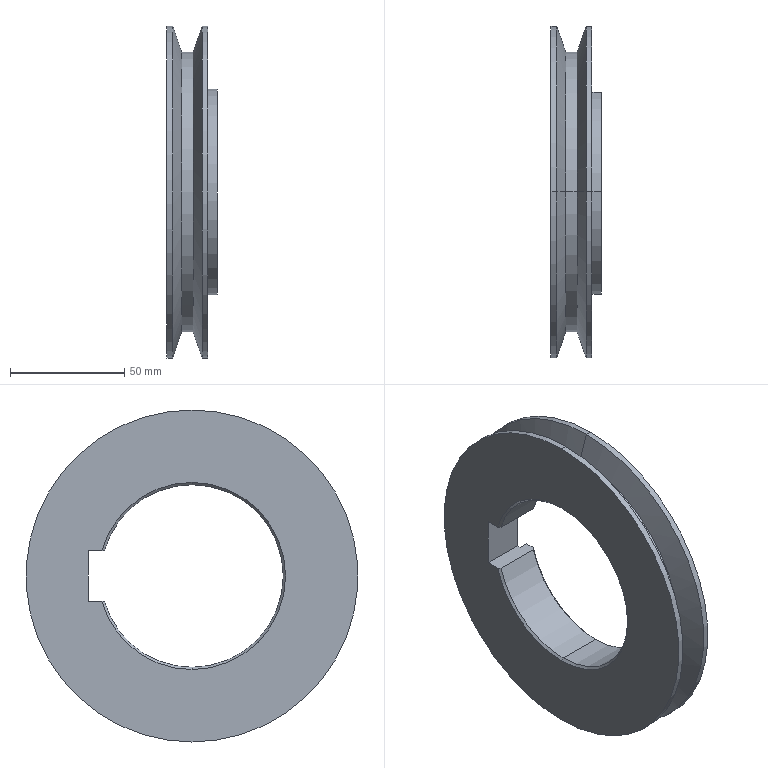Part | NX | features BREP 1 | 1 solid | 28 faces | box 22 x 145.5 x 145.5 mm | volume 167430 mm3 | cylinder 12 | cone 10 | plane 6 | commonest cylinder face diameters 145.5 x4 80 x3 90 x3 122.6 x2
STEP:
#1=CARTESIAN_POINT('',(1.,0.,-40.));
#2=VERTEX_POINT('',#1);
#3=CARTESIAN_POINT('',(1.,0.,40.));
#4=VERTEX_POINT('',#3);
#5=CARTESIAN_POINT('',(1.,0.,0.));
#6=DIRECTION('',(-1.,0.,0.));
#7=DIRECTION('',(0.,0.,-1.));
#8=AXIS2_PLACEMENT_3D('',#5,#6,#7);
#9=CIRCLE('',#8,40.);
#10=EDGE_CURVE('',#2,#4,#9,.T.);
#11=ORIENTED_EDGE('',*,*,#10,.F.);
#12=CARTESIAN_POINT('',(0.,0.,-41.));
#13=VERTEX_POINT('',#12);
#14=CARTESIAN_POINT('',(1.,0.,-40.));
#15=DIRECTION('',(-0.7071,0.,-0.7071));
#16=VECTOR('',#15,1000.);
#17=LINE('',#14,#16);
#18=EDGE_CURVE('',#2,#13,#17,.T.);
#19=ORIENTED_EDGE('',*,*,#18,.T.);
#20=CARTESIAN_POINT('',(0.,0.,41.));
#21=VERTEX_POINT('',#20);
#22=CARTESIAN_POINT('',(0.,0.,0.));
#23=DIRECTION('',(1.,0.,0.));
#24=DIRECTION('',(0.,0.,-1.));
#25=AXIS2_PLACEMENT_3D('',#22,#23,#24);
#26=CIRCLE('',#25,41.);
#27=EDGE_CURVE('',#21,#13,#26,.T.);
#28=ORIENTED_EDGE('',*,*,#27,.F.);
#29=CARTESIAN_POINT('',(1.,0.,40.));
#30=DIRECTION('',(-0.7071,0.,0.7071));
#31=VECTOR('',#30,1000.);
#32=LINE('',#29,#31);
#33=EDGE_CURVE('',#4,#21,#32,.T.);
#34=ORIENTED_EDGE('',*,*,#33,.F.);
#35=EDGE_LOOP('',(#11,#19,#28,#34));
#36=FACE_BOUND('',#35,.T.);
#37=CARTESIAN_POINT('',(1.,0.,0.));
#38=DIRECTION('',(-1.,0.,0.));
#39=DIRECTION('',(0.,0.,-1.));
#40=AXIS2_PLACEMENT_3D('',#37,#38,#39);
#41=CONICAL_SURFACE('',#40,40.,0.7854);
#42=ADVANCED_FACE('',(#36),#41,.F.);
#43=CARTESIAN_POINT('',(1.,38.458,11.));
#44=VERTEX_POINT('',#43);
#45=CARTESIAN_POINT('',(1.,0.,0.));
#46=DIRECTION('',(-1.,0.,0.));
#47=DIRECTION('',(0.,0.,-1.));
#48=AXIS2_PLACEMENT_3D('',#45,#46,#47);
#49=CIRCLE('',#48,40.);
#50=EDGE_CURVE('',#4,#44,#49,.T.);
#51=ORIENTED_EDGE('',*,*,#50,.F.);
#52=ORIENTED_EDGE('',*,*,#33,.T.);
#53=CARTESIAN_POINT('',(0.,39.497,11.));
#54=VERTEX_POINT('',#53);
#55=CARTESIAN_POINT('',(0.,0.,0.));
#56=DIRECTION('',(1.,0.,0.));
#57=DIRECTION('',(0.,0.,-1.));
#58=AXIS2_PLACEMENT_3D('',#55,#56,#57);
#59=CIRCLE('',#58,41.);
#60=EDGE_CURVE('',#54,#21,#59,.T.);
#61=ORIENTED_EDGE('',*,*,#60,.F.);
#62=CARTESIAN_POINT('',(1.,38.458,11.));
#63=CARTESIAN_POINT('',(0.6668,38.804,11.));
#64=CARTESIAN_POINT('',(0.3335,39.151,11.));
#65=CARTESIAN_POINT('',(0.,39.497,11.));
#66=B_SPLINE_CURVE_WITH_KNOTS('',3,(#62,#63,#64,#65),.UNSPECIFIED.,.F.,.F.,(4,4),(0.,1.),.PIECEWISE_BEZIER_KNOTS.);
#67=EDGE_CURVE('',#44,#54,#66,.T.);
#68=ORIENTED_EDGE('',*,*,#67,.F.);
#69=EDGE_LOOP('',(#51,#52,#61,#68));
#70=FACE_BOUND('',#69,.T.);
#71=CARTESIAN_POINT('',(1.,0.,0.));
#72=DIRECTION('',(-1.,0.,0.));
#73=DIRECTION('',(0.,0.,-1.));
#74=AXIS2_PLACEMENT_3D('',#71,#72,#73);
#75=CONICAL_SURFACE('',#74,40.,0.7854);
#76=ADVANCED_FACE('',(#70),#75,.F.);
#77=CARTESIAN_POINT('',(21.,0.,40.));
#78=VERTEX_POINT('',#77);
#79=CARTESIAN_POINT('',(21.,0.,-40.));
#80=VERTEX_POINT('',#79);
#81=CARTESIAN_POINT('',(21.,0.,0.));
#82=DIRECTION('',(1.,0.,0.));
#83=DIRECTION('',(0.,0.,1.));
#84=AXIS2_PLACEMENT_3D('',#81,#82,#83);
#85=CIRCLE('',#84,40.);
#86=EDGE_CURVE('',#78,#80,#85,.T.);
#87=ORIENTED_EDGE('',*,*,#86,.F.);
#88=CARTESIAN_POINT('',(22.,0.,41.));
#89=VERTEX_POINT('',#88);
#90=CARTESIAN_POINT('',(22.,0.,41.));
#91=DIRECTION('',(0.7071,0.,0.7071));
#92=VECTOR('',#91,1000.);
#93=LINE('',#90,#92);
#94=EDGE_CURVE('',#78,#89,#93,.T.);
#95=ORIENTED_EDGE('',*,*,#94,.T.);
#96=CARTESIAN_POINT('',(22.,0.,-41.));
#97=VERTEX_POINT('',#96);
#98=CARTESIAN_POINT('',(22.,0.,0.));
#99=DIRECTION('',(-1.,0.,0.));
#100=DIRECTION('',(0.,0.,1.));
#101=AXIS2_PLACEMENT_3D('',#98,#99,#100);
#102=CIRCLE('',#101,41.);
#103=EDGE_CURVE('',#97,#89,#102,.T.);
#104=ORIENTED_EDGE('',*,*,#103,.F.);
#105=CARTESIAN_POINT('',(22.,0.,-41.));
#106=DIRECTION('',(0.7071,0.,-0.7071));
#107=VECTOR('',#106,1000.);
#108=LINE('',#105,#107);
#109=EDGE_CURVE('',#80,#97,#108,.T.);
#110=ORIENTED_EDGE('',*,*,#109,.F.);
#111=EDGE_LOOP('',(#87,#95,#104,#110));
#112=FACE_BOUND('',#111,.T.);
#113=CARTESIAN_POINT('',(22.,0.,0.));
#114=DIRECTION('',(1.,0.,0.));
#115=DIRECTION('',(0.,0.,1.));
#116=AXIS2_PLACEMENT_3D('',#113,#114,#115);
#117=CONICAL_SURFACE('',#116,41.,0.7854);
#118=ADVANCED_FACE('',(#112),#117,.F.);
#119=CARTESIAN_POINT('',(21.,38.458,-11.));
#120=VERTEX_POINT('',#119);
#121=CARTESIAN_POINT('',(21.,0.,0.));
#122=DIRECTION('',(1.,0.,0.));
#123=DIRECTION('',(0.,0.,1.));
#124=AXIS2_PLACEMENT_3D('',#121,#122,#123);
#125=CIRCLE('',#124,40.);
#126=EDGE_CURVE('',#80,#120,#125,.T.);
#127=ORIENTED_EDGE('',*,*,#126,.F.);
#128=ORIENTED_EDGE('',*,*,#109,.T.);
#129=CARTESIAN_POINT('',(22.,39.497,-11.));
#130=VERTEX_POINT('',#129);
#131=CARTESIAN_POINT('',(22.,0.,0.));
#132=DIRECTION('',(-1.,0.,0.));
#133=DIRECTION('',(0.,0.,1.));
#134=AXIS2_PLACEMENT_3D('',#131,#132,#133);
#135=CIRCLE('',#134,41.);
#136=EDGE_CURVE('',#130,#97,#135,.T.);
#137=ORIENTED_EDGE('',*,*,#136,.F.);
#138=CARTESIAN_POINT('',(21.,38.458,-11.));
#139=CARTESIAN_POINT('',(21.333,38.804,-11.));
#140=CARTESIAN_POINT('',(21.666,39.151,-11.));
#141=CARTESIAN_POINT('',(22.,39.497,-11.));
#142=B_SPLINE_CURVE_WITH_KNOTS('',3,(#138,#139,#140,#141),.UNSPECIFIED.,.F.,.F.,(4,4),(0.,1.),.PIECEWISE_BEZIER_KNOTS.);
#143=EDGE_CURVE('',#120,#130,#142,.T.);
#144=ORIENTED_EDGE('',*,*,#143,.F.);
#145=EDGE_LOOP('',(#127,#128,#137,#144));
#146=FACE_BOUND('',#145,.T.);
#147=CARTESIAN_POINT('',(22.,0.,0.));
#148=DIRECTION('',(1.,0.,0.));
#149=DIRECTION('',(0.,0.,1.));
#150=AXIS2_PLACEMENT_3D('',#147,#148,#149);
#151=CONICAL_SURFACE('',#150,41.,0.7854);
#152=ADVANCED_FACE('',(#146),#151,.F.);
#153=CARTESIAN_POINT('',(6.496,0.,61.3));
#154=VERTEX_POINT('',#153);
#155=CARTESIAN_POINT('',(6.496,0.,-61.3));
#156=VERTEX_POINT('',#155);
#157=CARTESIAN_POINT('',(6.496,0.,0.));
#158=DIRECTION('',(-1.,0.,0.));
#159=DIRECTION('',(0.,0.,1.));
#160=AXIS2_PLACEMENT_3D('',#157,#158,#159);
#161=CIRCLE('',#160,61.3);
#162=EDGE_CURVE('',#154,#156,#161,.T.);
#163=ORIENTED_EDGE('',*,*,#162,.T.);
#164=CARTESIAN_POINT('',(2.553,0.,-72.75));
#165=VERTEX_POINT('',#164);
#166=CARTESIAN_POINT('',(2.553,0.,-72.75));
#167=DIRECTION('',(-0.3256,0.,-0.9455));
#168=VECTOR('',#167,1000.);
#169=LINE('',#166,#168);
#170=EDGE_CURVE('',#156,#165,#169,.T.);
#171=ORIENTED_EDGE('',*,*,#170,.T.);
#172=CARTESIAN_POINT('',(2.553,0.,72.75));
#173=VERTEX_POINT('',#172);
#174=CARTESIAN_POINT('',(2.553,0.,0.));
#175=DIRECTION('',(-1.,0.,0.));
#176=DIRECTION('',(0.,0.,1.));
#177=AXIS2_PLACEMENT_3D('',#174,#175,#176);
#178=CIRCLE('',#177,72.75);
#179=EDGE_CURVE('',#173,#165,#178,.T.);
#180=ORIENTED_EDGE('',*,*,#179,.F.);
#181=CARTESIAN_POINT('',(2.553,0.,72.75));
#182=DIRECTION('',(-0.3256,0.,0.9455));
#183=VECTOR('',#182,1000.);
#184=LINE('',#181,#183);
#185=EDGE_CURVE('',#154,#173,#184,.T.);
#186=ORIENTED_EDGE('',*,*,#185,.F.);
#187=EDGE_LOOP('',(#163,#171,#180,#186));
#188=FACE_BOUND('',#187,.T.);
#189=CARTESIAN_POINT('',(2.553,0.,0.));
#190=DIRECTION('',(-1.,0.,0.));
#191=DIRECTION('',(0.,0.,-1.));
#192=AXIS2_PLACEMENT_3D('',#189,#190,#191);
#193=CONICAL_SURFACE('',#192,72.75,1.239);
#194=ADVANCED_FACE('',(#188),#193,.T.);
#195=CARTESIAN_POINT('',(11.504,0.,61.3));
#196=VERTEX_POINT('',#195);
#197=CARTESIAN_POINT('',(11.504,0.,-61.3));
#198=VERTEX_POINT('',#197);
#199=CARTESIAN_POINT('',(11.504,0.,0.));
#200=DIRECTION('',(-1.,0.,0.));
#201=DIRECTION('',(0.,0.,1.));
#202=AXIS2_PLACEMENT_3D('',#199,#200,#201);
#203=CIRCLE('',#202,61.3);
#204=EDGE_CURVE('',#196,#198,#203,.T.);
#205=ORIENTED_EDGE('',*,*,#204,.F.);
#206=CARTESIAN_POINT('',(15.447,0.,72.75));
#207=VERTEX_POINT('',#206);
#208=CARTESIAN_POINT('',(11.504,0.,61.3));
#209=DIRECTION('',(0.3256,0.,0.9455));
#210=VECTOR('',#209,1000.);
#211=LINE('',#208,#210);
#212=EDGE_CURVE('',#207,#196,#211,.F.);
#213=ORIENTED_EDGE('',*,*,#212,.F.);
#214=CARTESIAN_POINT('',(15.447,0.,-72.75));
#215=VERTEX_POINT('',#214);
#216=CARTESIAN_POINT('',(15.447,0.,0.));
#217=DIRECTION('',(-1.,0.,0.));
#218=DIRECTION('',(0.,0.,1.));
#219=AXIS2_PLACEMENT_3D('',#216,#217,#218);
#220=CIRCLE('',#219,72.75);
#221=EDGE_CURVE('',#207,#215,#220,.T.);
#222=ORIENTED_EDGE('',*,*,#221,.T.);
#223=CARTESIAN_POINT('',(11.504,0.,-61.3));
#224=DIRECTION('',(0.3256,0.,-0.9455));
#225=VECTOR('',#224,1000.);
#226=LINE('',#223,#225);
#227=EDGE_CURVE('',#215,#198,#226,.F.);
#228=ORIENTED_EDGE('',*,*,#227,.T.);
#229=EDGE_LOOP('',(#205,#213,#222,#228));
#230=FACE_BOUND('',#229,.T.);
#231=CARTESIAN_POINT('',(11.504,0.,0.));
#232=DIRECTION('',(1.,0.,0.));
#233=DIRECTION('',(0.,0.,1.));
#234=AXIS2_PLACEMENT_3D('',#231,#232,#233);
#235=CONICAL_SURFACE('',#234,61.3,1.239);
#236=ADVANCED_FACE('',(#230),#235,.T.);
#237=ORIENTED_EDGE('',*,*,#204,.T.);
#238=CARTESIAN_POINT('',(0.,0.,-61.3));
#239=DIRECTION('',(-1.,0.,0.));
#240=VECTOR('',#239,1000.);
#241=LINE('',#238,#240);
#242=EDGE_CURVE('',#198,#156,#241,.T.);
#243=ORIENTED_EDGE('',*,*,#242,.T.);
#244=ORIENTED_EDGE('',*,*,#162,.F.);
#245=CARTESIAN_POINT('',(0.,0.,61.3));
#246=DIRECTION('',(-1.,0.,0.));
#247=VECTOR('',#246,1000.);
#248=LINE('',#245,#247);
#249=EDGE_CURVE('',#196,#154,#248,.T.);
#250=ORIENTED_EDGE('',*,*,#249,.F.);
#251=EDGE_LOOP('',(#237,#243,#244,#250));
#252=FACE_BOUND('',#251,.T.);
#253=CARTESIAN_POINT('',(0.,0.,0.));
#254=DIRECTION('',(-1.,0.,0.));
#255=DIRECTION('',(0.,0.,-1.));
#256=AXIS2_PLACEMENT_3D('',#253,#254,#255);
#257=CYLINDRICAL_SURFACE('',#256,61.3);
#258=ADVANCED_FACE('',(#252),#257,.T.);
#259=CARTESIAN_POINT('',(22.,43.635,-11.));
#260=VERTEX_POINT('',#259);
#261=CARTESIAN_POINT('',(22.,0.,-45.));
#262=VERTEX_POINT('',#261);
#263=CARTESIAN_POINT('',(22.,0.,0.));
#264=DIRECTION('',(-1.,0.,0.));
#265=DIRECTION('',(0.,0.,1.));
#266=AXIS2_PLACEMENT_3D('',#263,#264,#265);
#267=CIRCLE('',#266,45.);
#268=EDGE_CURVE('',#260,#262,#267,.T.);
#269=ORIENTED_EDGE('',*,*,#268,.T.);
#270=CARTESIAN_POINT('',(18.,0.,-45.));
#271=VERTEX_POINT('',#270);
#272=CARTESIAN_POINT('',(0.,0.,-45.));
#273=DIRECTION('',(-1.,0.,0.));
#274=VECTOR('',#273,1000.);
#275=LINE('',#272,#274);
#276=EDGE_CURVE('',#262,#271,#275,.T.);
#277=ORIENTED_EDGE('',*,*,#276,.T.);
#278=CARTESIAN_POINT('',(18.,43.635,-11.));
#279=VERTEX_POINT('',#278);
#280=CARTESIAN_POINT('',(18.,0.,0.));
#281=DIRECTION('',(-1.,0.,0.));
#282=DIRECTION('',(0.,0.,1.));
#283=AXIS2_PLACEMENT_3D('',#280,#281,#282);
#284=CIRCLE('',#283,45.);
#285=EDGE_CURVE('',#279,#271,#284,.T.);
#286=ORIENTED_EDGE('',*,*,#285,.F.);
#287=CARTESIAN_POINT('',(0.,43.635,-11.));
#288=DIRECTION('',(1.,0.,0.));
#289=VECTOR('',#288,1000.);
#290=LINE('',#287,#289);
#291=EDGE_CURVE('',#279,#260,#290,.T.);
#292=ORIENTED_EDGE('',*,*,#291,.T.);
#293=EDGE_LOOP('',(#269,#277,#286,#292));
#294=FACE_BOUND('',#293,.T.);
#295=CARTESIAN_POINT('',(0.,0.,0.));
#296=DIRECTION('',(-1.,0.,0.));
#297=DIRECTION('',(0.,0.,-1.));
#298=AXIS2_PLACEMENT_3D('',#295,#296,#297);
#299=CYLINDRICAL_SURFACE('',#298,45.);
#300=ADVANCED_FACE('',(#294),#299,.T.);
#301=ORIENTED_EDGE('',*,*,#276,.F.);
#302=CARTESIAN_POINT('',(22.,0.,45.));
#303=VERTEX_POINT('',#302);
#304=CARTESIAN_POINT('',(22.,0.,0.));
#305=DIRECTION('',(-1.,0.,0.));
#306=DIRECTION('',(0.,0.,1.));
#307=AXIS2_PLACEMENT_3D('',#304,#305,#306);
#308=CIRCLE('',#307,45.);
#309=EDGE_CURVE('',#262,#303,#308,.T.);
#310=ORIENTED_EDGE('',*,*,#309,.T.);
#311=CARTESIAN_POINT('',(18.,0.,45.));
#312=VERTEX_POINT('',#311);
#313=CARTESIAN_POINT('',(0.,0.,45.));
#314=DIRECTION('',(-1.,0.,0.));
#315=VECTOR('',#314,1000.);
#316=LINE('',#313,#315);
#317=EDGE_CURVE('',#303,#312,#316,.T.);
#318=ORIENTED_EDGE('',*,*,#317,.T.);
#319=CARTESIAN_POINT('',(18.,0.,0.));
#320=DIRECTION('',(-1.,0.,0.));
#321=DIRECTION('',(0.,0.,1.));
#322=AXIS2_PLACEMENT_3D('',#319,#320,#321);
#323=CIRCLE('',#322,45.);
#324=EDGE_CURVE('',#271,#312,#323,.T.);
#325=ORIENTED_EDGE('',*,*,#324,.F.);
#326=EDGE_LOOP('',(#301,#310,#318,#325));
#327=FACE_BOUND('',#326,.T.);
#328=CARTESIAN_POINT('',(0.,0.,0.));
#329=DIRECTION('',(-1.,0.,0.));
#330=DIRECTION('',(0.,0.,-1.));
#331=AXIS2_PLACEMENT_3D('',#328,#329,#330);
#332=CYLINDRICAL_SURFACE('',#331,45.);
#333=ADVANCED_FACE('',(#327),#332,.T.);
#334=ORIENTED_EDGE('',*,*,#86,.T.);
#335=CARTESIAN_POINT('',(0.,0.,-40.));
#336=DIRECTION('',(-1.,0.,0.));
#337=VECTOR('',#336,1000.);
#338=LINE('',#335,#337);
#339=EDGE_CURVE('',#80,#2,#338,.T.);
#340=ORIENTED_EDGE('',*,*,#339,.T.);
#341=ORIENTED_EDGE('',*,*,#10,.T.);
#342=CARTESIAN_POINT('',(0.,0.,40.));
#343=DIRECTION('',(-1.,0.,0.));
#344=VECTOR('',#343,1000.);
#345=LINE('',#342,#344);
#346=EDGE_CURVE('',#78,#4,#345,.T.);
#347=ORIENTED_EDGE('',*,*,#346,.F.);
#348=EDGE_LOOP('',(#334,#340,#341,#347));
#349=FACE_BOUND('',#348,.T.);
#350=CARTESIAN_POINT('',(0.,0.,0.));
#351=DIRECTION('',(-1.,0.,0.));
#352=DIRECTION('',(0.,0.,-1.));
#353=AXIS2_PLACEMENT_3D('',#350,#351,#352);
#354=CYLINDRICAL_SURFACE('',#353,40.);
#355=ADVANCED_FACE('',(#349),#354,.F.);
#356=CARTESIAN_POINT('',(21.,38.458,11.));
#357=VERTEX_POINT('',#356);
#358=CARTESIAN_POINT('',(21.,0.,0.));
#359=DIRECTION('',(1.,0.,0.));
#360=DIRECTION('',(0.,0.,1.));
#361=AXIS2_PLACEMENT_3D('',#358,#359,#360);
#362=CIRCLE('',#361,40.);
#363=EDGE_CURVE('',#357,#78,#362,.T.);
#364=ORIENTED_EDGE('',*,*,#363,.T.);
#365=ORIENTED_EDGE('',*,*,#346,.T.);
#366=ORIENTED_EDGE('',*,*,#50,.T.);
#367=CARTESIAN_POINT('',(22.,38.458,11.));
#368=DIRECTION('',(-1.,0.,0.));
#369=VECTOR('',#368,1000.);
#370=LINE('',#367,#369);
#371=EDGE_CURVE('',#357,#44,#370,.T.);
#372=ORIENTED_EDGE('',*,*,#371,.F.);
#373=EDGE_LOOP('',(#364,#365,#366,#372));
#374=FACE_BOUND('',#373,.T.);
#375=CARTESIAN_POINT('',(0.,0.,0.));
#376=DIRECTION('',(-1.,0.,0.));
#377=DIRECTION('',(0.,0.,-1.));
#378=AXIS2_PLACEMENT_3D('',#375,#376,#377);
#379=CYLINDRICAL_SURFACE('',#378,40.);
#380=ADVANCED_FACE('',(#374),#379,.F.);
#381=ORIENTED_EDGE('',*,*,#179,.T.);
#382=CARTESIAN_POINT('',(0.,0.,-72.75));
#383=VERTEX_POINT('',#382);
#384=CARTESIAN_POINT('',(0.,0.,-72.75));
#385=DIRECTION('',(-1.,0.,0.));
#386=VECTOR('',#385,1000.);
#387=LINE('',#384,#386);
#388=EDGE_CURVE('',#165,#383,#387,.T.);
#389=ORIENTED_EDGE('',*,*,#388,.T.);
#390=CARTESIAN_POINT('',(0.,0.,72.75));
#391=VERTEX_POINT('',#390);
#392=CARTESIAN_POINT('',(0.,0.,0.));
#393=DIRECTION('',(-1.,0.,0.));
#394=DIRECTION('',(0.,0.,1.));
#395=AXIS2_PLACEMENT_3D('',#392,#393,#394);
#396=CIRCLE('',#395,72.75);
#397=EDGE_CURVE('',#391,#383,#396,.T.);
#398=ORIENTED_EDGE('',*,*,#397,.F.);
#399=CARTESIAN_POINT('',(0.,0.,72.75));
#400=DIRECTION('',(-1.,0.,0.));
#401=VECTOR('',#400,1000.);
#402=LINE('',#399,#401);
#403=EDGE_CURVE('',#173,#391,#402,.T.);
#404=ORIENTED_EDGE('',*,*,#403,.F.);
#405=EDGE_LOOP('',(#381,#389,#398,#404));
#406=FACE_BOUND('',#405,.T.);
#407=CARTESIAN_POINT('',(0.,0.,0.));
#408=DIRECTION('',(-1.,0.,0.));
#409=DIRECTION('',(0.,0.,-1.));
#410=AXIS2_PLACEMENT_3D('',#407,#408,#409);
#411=CYLINDRICAL_SURFACE('',#410,72.75);
#412=ADVANCED_FACE('',(#406),#411,.T.);
#413=CARTESIAN_POINT('',(18.,0.,72.75));
#414=VERTEX_POINT('',#413);
#415=CARTESIAN_POINT('',(18.,0.,-72.75));
#416=VERTEX_POINT('',#415);
#417=CARTESIAN_POINT('',(18.,0.,0.));
#418=DIRECTION('',(-1.,0.,0.));
#419=DIRECTION('',(0.,0.,1.));
#420=AXIS2_PLACEMENT_3D('',#417,#418,#419);
#421=CIRCLE('',#420,72.75);
#422=EDGE_CURVE('',#414,#416,#421,.T.);
#423=ORIENTED_EDGE('',*,*,#422,.T.);
#424=CARTESIAN_POINT('',(0.,0.,-72.75));
#425=DIRECTION('',(-1.,0.,0.));
#426=VECTOR('',#425,1000.);
#427=LINE('',#424,#426);
#428=EDGE_CURVE('',#416,#215,#427,.T.);
#429=ORIENTED_EDGE('',*,*,#428,.T.);
#430=ORIENTED_EDGE('',*,*,#221,.F.);
#431=CARTESIAN_POINT('',(0.,0.,72.75));
#432=DIRECTION('',(-1.,0.,0.));
#433=VECTOR('',#432,1000.);
#434=LINE('',#431,#433);
#435=EDGE_CURVE('',#414,#207,#434,.T.);
#436=ORIENTED_EDGE('',*,*,#435,.F.);
#437=EDGE_LOOP('',(#423,#429,#430,#436));
#438=FACE_BOUND('',#437,.T.);
#439=CARTESIAN_POINT('',(0.,0.,0.));
#440=DIRECTION('',(-1.,0.,0.));
#441=DIRECTION('',(0.,0.,-1.));
#442=AXIS2_PLACEMENT_3D('',#439,#440,#441);
#443=CYLINDRICAL_SURFACE('',#442,72.75);
#444=ADVANCED_FACE('',(#438),#443,.T.);
#445=ORIENTED_EDGE('',*,*,#428,.F.);
#446=CARTESIAN_POINT('',(18.,0.,0.));
#447=DIRECTION('',(-1.,0.,0.));
#448=DIRECTION('',(0.,0.,1.));
#449=AXIS2_PLACEMENT_3D('',#446,#447,#448);
#450=CIRCLE('',#449,72.75);
#451=EDGE_CURVE('',#416,#414,#450,.T.);
#452=ORIENTED_EDGE('',*,*,#451,.T.);
#453=ORIENTED_EDGE('',*,*,#435,.T.);
#454=CARTESIAN_POINT('',(15.447,0.,0.));
#455=DIRECTION('',(-1.,0.,0.));
#456=DIRECTION('',(0.,0.,1.));
#457=AXIS2_PLACEMENT_3D('',#454,#455,#456);
#458=CIRCLE('',#457,72.75);
#459=EDGE_CURVE('',#215,#207,#458,.T.);
#460=ORIENTED_EDGE('',*,*,#459,.F.);
#461=EDGE_LOOP('',(#445,#452,#453,#460));
#462=FACE_BOUND('',#461,.T.);
#463=CARTESIAN_POINT('',(0.,0.,0.));
#464=DIRECTION('',(-1.,0.,0.));
#465=DIRECTION('',(0.,0.,-1.));
#466=AXIS2_PLACEMENT_3D('',#463,#464,#465);
#467=CYLINDRICAL_SURFACE('',#466,72.75);
#468=ADVANCED_FACE('',(#462),#467,.T.);
#469=ORIENTED_EDGE('',*,*,#388,.F.);
#470=CARTESIAN_POINT('',(2.553,0.,0.));
#471=DIRECTION('',(-1.,0.,0.));
#472=DIRECTION('',(0.,0.,1.));
#473=AXIS2_PLACEMENT_3D('',#470,#471,#472);
#474=CIRCLE('',#473,72.75);
#475=EDGE_CURVE('',#165,#173,#474,.T.);
#476=ORIENTED_EDGE('',*,*,#475,.T.);
#477=ORIENTED_EDGE('',*,*,#403,.T.);
#478=CARTESIAN_POINT('',(0.,0.,0.));
#479=DIRECTION('',(-1.,0.,0.));
#480=DIRECTION('',(0.,0.,1.));
#481=AXIS2_PLACEMENT_3D('',#478,#479,#480);
#482=CIRCLE('',#481,72.75);
#483=EDGE_CURVE('',#383,#391,#482,.T.);
#484=ORIENTED_EDGE('',*,*,#483,.F.);
#485=EDGE_LOOP('',(#469,#476,#477,#484));
#486=FACE_BOUND('',#485,.T.);
#487=CARTESIAN_POINT('',(0.,0.,0.));
#488=DIRECTION('',(-1.,0.,0.));
#489=DIRECTION('',(0.,0.,-1.));
#490=AXIS2_PLACEMENT_3D('',#487,#488,#489);
#491=CYLINDRICAL_SURFACE('',#490,72.75);
#492=ADVANCED_FACE('',(#486),#491,.T.);
#493=ORIENTED_EDGE('',*,*,#339,.F.);
#494=ORIENTED_EDGE('',*,*,#126,.T.);
#495=CARTESIAN_POINT('',(1.,38.458,-11.));
#496=VERTEX_POINT('',#495);
#497=CARTESIAN_POINT('',(22.,38.458,-11.));
#498=DIRECTION('',(-1.,0.,0.));
#499=VECTOR('',#498,1000.);
#500=LINE('',#497,#499);
#501=EDGE_CURVE('',#120,#496,#500,.T.);
#502=ORIENTED_EDGE('',*,*,#501,.T.);
#503=CARTESIAN_POINT('',(1.,0.,0.));
#504=DIRECTION('',(-1.,0.,0.));
#505=DIRECTION('',(0.,0.,-1.));
#506=AXIS2_PLACEMENT_3D('',#503,#504,#505);
#507=CIRCLE('',#506,40.);
#508=EDGE_CURVE('',#496,#2,#507,.T.);
#509=ORIENTED_EDGE('',*,*,#508,.T.);
#510=EDGE_LOOP('',(#493,#494,#502,#509));
#511=FACE_BOUND('',#510,.T.);
#512=CARTESIAN_POINT('',(0.,0.,0.));
#513=DIRECTION('',(-1.,0.,0.));
#514=DIRECTION('',(0.,0.,-1.));
#515=AXIS2_PLACEMENT_3D('',#512,#513,#514);
#516=CYLINDRICAL_SURFACE('',#515,40.);
#517=ADVANCED_FACE('',(#511),#516,.F.);
#518=ORIENTED_EDGE('',*,*,#268,.F.);
#519=CARTESIAN_POINT('',(22.,38.458,-11.));
#520=DIRECTION('',(0.,-1.,0.));
#521=VECTOR('',#520,1000.);
#522=LINE('',#519,#521);
#523=EDGE_CURVE('',#260,#130,#522,.T.);
#524=ORIENTED_EDGE('',*,*,#523,.T.);
#525=ORIENTED_EDGE('',*,*,#136,.T.);
#526=ORIENTED_EDGE('',*,*,#103,.T.);
#527=CARTESIAN_POINT('',(22.,39.497,11.));
#528=VERTEX_POINT('',#527);
#529=CARTESIAN_POINT('',(22.,0.,0.));
#530=DIRECTION('',(-1.,0.,0.));
#531=DIRECTION('',(0.,0.,1.));
#532=AXIS2_PLACEMENT_3D('',#529,#530,#531);
#533=CIRCLE('',#532,41.);
#534=EDGE_CURVE('',#89,#528,#533,.T.);
#535=ORIENTED_EDGE('',*,*,#534,.T.);
#536=CARTESIAN_POINT('',(22.,43.635,11.));
#537=VERTEX_POINT('',#536);
#538=CARTESIAN_POINT('',(22.,38.458,11.));
#539=DIRECTION('',(0.,1.,0.));
#540=VECTOR('',#539,1000.);
#541=LINE('',#538,#540);
#542=EDGE_CURVE('',#528,#537,#541,.T.);
#543=ORIENTED_EDGE('',*,*,#542,.T.);
#544=CARTESIAN_POINT('',(22.,0.,0.));
#545=DIRECTION('',(-1.,0.,0.));
#546=DIRECTION('',(0.,0.,1.));
#547=AXIS2_PLACEMENT_3D('',#544,#545,#546);
#548=CIRCLE('',#547,45.);
#549=EDGE_CURVE('',#303,#537,#548,.T.);
#550=ORIENTED_EDGE('',*,*,#549,.F.);
#551=ORIENTED_EDGE('',*,*,#309,.F.);
#552=EDGE_LOOP('',(#518,#524,#525,#526,#535,#543,#550,#551));
#553=FACE_BOUND('',#552,.T.);
#554=CARTESIAN_POINT('',(22.,45.,0.));
#555=DIRECTION('',(-1.,0.,0.));
#556=DIRECTION('',(0.,-1.,0.));
#557=AXIS2_PLACEMENT_3D('',#554,#555,#556);
#558=PLANE('',#557);
#559=ADVANCED_FACE('',(#553),#558,.F.);
#560=ORIENTED_EDGE('',*,*,#317,.F.);
#561=ORIENTED_EDGE('',*,*,#549,.T.);
#562=CARTESIAN_POINT('',(18.,43.635,11.));
#563=VERTEX_POINT('',#562);
#564=CARTESIAN_POINT('',(0.,43.635,11.));
#565=DIRECTION('',(-1.,0.,0.));
#566=VECTOR('',#565,1000.);
#567=LINE('',#564,#566);
#568=EDGE_CURVE('',#537,#563,#567,.T.);
#569=ORIENTED_EDGE('',*,*,#568,.T.);
#570=CARTESIAN_POINT('',(18.,0.,0.));
#571=DIRECTION('',(-1.,0.,0.));
#572=DIRECTION('',(0.,0.,1.));
#573=AXIS2_PLACEMENT_3D('',#570,#571,#572);
#574=CIRCLE('',#573,45.);
#575=EDGE_CURVE('',#312,#563,#574,.T.);
#576=ORIENTED_EDGE('',*,*,#575,.F.);
#577=EDGE_LOOP('',(#560,#561,#569,#576));
#578=FACE_BOUND('',#577,.T.);
#579=CARTESIAN_POINT('',(0.,0.,0.));
#580=DIRECTION('',(-1.,0.,0.));
#581=DIRECTION('',(0.,0.,-1.));
#582=AXIS2_PLACEMENT_3D('',#579,#580,#581);
#583=CYLINDRICAL_SURFACE('',#582,45.);
#584=ADVANCED_FACE('',(#578),#583,.T.);
#585=ORIENTED_EDGE('',*,*,#422,.F.);
#586=ORIENTED_EDGE('',*,*,#451,.F.);
#587=EDGE_LOOP('',(#585,#586));
#588=FACE_BOUND('',#587,.T.);
#589=CARTESIAN_POINT('',(18.,45.4,11.));
#590=VERTEX_POINT('',#589);
#591=CARTESIAN_POINT('',(18.,45.4,-11.));
#592=VERTEX_POINT('',#591);
#593=CARTESIAN_POINT('',(18.,45.4,0.));
#594=DIRECTION('',(0.,0.,-1.));
#595=VECTOR('',#594,1000.);
#596=LINE('',#593,#595);
#597=EDGE_CURVE('',#590,#592,#596,.T.);
#598=ORIENTED_EDGE('',*,*,#597,.T.);
#599=CARTESIAN_POINT('',(18.,72.75,-11.));
#600=DIRECTION('',(0.,-1.,0.));
#601=VECTOR('',#600,1000.);
#602=LINE('',#599,#601);
#603=EDGE_CURVE('',#592,#279,#602,.T.);
#604=ORIENTED_EDGE('',*,*,#603,.T.);
#605=ORIENTED_EDGE('',*,*,#285,.T.);
#606=ORIENTED_EDGE('',*,*,#324,.T.);
#607=ORIENTED_EDGE('',*,*,#575,.T.);
#608=CARTESIAN_POINT('',(18.,72.75,11.));
#609=DIRECTION('',(0.,1.,0.));
#610=VECTOR('',#609,1000.);
#611=LINE('',#608,#610);
#612=EDGE_CURVE('',#563,#590,#611,.T.);
#613=ORIENTED_EDGE('',*,*,#612,.T.);
#614=EDGE_LOOP('',(#598,#604,#605,#606,#607,#613));
#615=FACE_BOUND('',#614,.T.);
#616=CARTESIAN_POINT('',(18.,72.75,0.));
#617=DIRECTION('',(-1.,0.,0.));
#618=DIRECTION('',(0.,-1.,0.));
#619=AXIS2_PLACEMENT_3D('',#616,#617,#618);
#620=PLANE('',#619);
#621=ADVANCED_FACE('',(#588,#615),#620,.F.);
#622=ORIENTED_EDGE('',*,*,#397,.T.);
#623=ORIENTED_EDGE('',*,*,#483,.T.);
#624=EDGE_LOOP('',(#622,#623));
#625=FACE_BOUND('',#624,.T.);
#626=ORIENTED_EDGE('',*,*,#60,.T.);
#627=ORIENTED_EDGE('',*,*,#27,.T.);
#628=CARTESIAN_POINT('',(0.,39.497,-11.));
#629=VERTEX_POINT('',#628);
#630=CARTESIAN_POINT('',(0.,0.,0.));
#631=DIRECTION('',(1.,0.,0.));
#632=DIRECTION('',(0.,0.,-1.));
#633=AXIS2_PLACEMENT_3D('',#630,#631,#632);
#634=CIRCLE('',#633,41.);
#635=EDGE_CURVE('',#13,#629,#634,.T.);
#636=ORIENTED_EDGE('',*,*,#635,.T.);
#637=CARTESIAN_POINT('',(0.,45.4,-11.));
#638=VERTEX_POINT('',#637);
#639=CARTESIAN_POINT('',(0.,38.458,-11.));
#640=DIRECTION('',(0.,-1.,0.));
#641=VECTOR('',#640,1000.);
#642=LINE('',#639,#641);
#643=EDGE_CURVE('',#638,#629,#642,.T.);
#644=ORIENTED_EDGE('',*,*,#643,.F.);
#645=CARTESIAN_POINT('',(0.,45.4,11.));
#646=VERTEX_POINT('',#645);
#647=CARTESIAN_POINT('',(0.,45.4,-11.));
#648=DIRECTION('',(0.,0.,-1.));
#649=VECTOR('',#648,1000.);
#650=LINE('',#647,#649);
#651=EDGE_CURVE('',#646,#638,#650,.T.);
#652=ORIENTED_EDGE('',*,*,#651,.F.);
#653=CARTESIAN_POINT('',(0.,38.458,11.));
#654=DIRECTION('',(0.,1.,0.));
#655=VECTOR('',#654,1000.);
#656=LINE('',#653,#655);
#657=EDGE_CURVE('',#54,#646,#656,.T.);
#658=ORIENTED_EDGE('',*,*,#657,.F.);
#659=EDGE_LOOP('',(#626,#627,#636,#644,#652,#658));
#660=FACE_BOUND('',#659,.T.);
#661=CARTESIAN_POINT('',(0.,40.,0.));
#662=DIRECTION('',(1.,0.,0.));
#663=DIRECTION('',(0.,0.,1.));
#664=AXIS2_PLACEMENT_3D('',#661,#662,#663);
#665=PLANE('',#664);
#666=ADVANCED_FACE('',(#625,#660),#665,.F.);
#667=ORIENTED_EDGE('',*,*,#242,.F.);
#668=CARTESIAN_POINT('',(11.504,0.,0.));
#669=DIRECTION('',(-1.,0.,0.));
#670=DIRECTION('',(0.,0.,1.));
#671=AXIS2_PLACEMENT_3D('',#668,#669,#670);
#672=CIRCLE('',#671,61.3);
#673=EDGE_CURVE('',#198,#196,#672,.T.);
#674=ORIENTED_EDGE('',*,*,#673,.T.);
#675=ORIENTED_EDGE('',*,*,#249,.T.);
#676=CARTESIAN_POINT('',(6.496,0.,0.));
#677=DIRECTION('',(-1.,0.,0.));
#678=DIRECTION('',(0.,0.,1.));
#679=AXIS2_PLACEMENT_3D('',#676,#677,#678);
#680=CIRCLE('',#679,61.3);
#681=EDGE_CURVE('',#156,#154,#680,.T.);
#682=ORIENTED_EDGE('',*,*,#681,.F.);
#683=EDGE_LOOP('',(#667,#674,#675,#682));
#684=FACE_BOUND('',#683,.T.);
#685=CARTESIAN_POINT('',(0.,0.,0.));
#686=DIRECTION('',(-1.,0.,0.));
#687=DIRECTION('',(0.,0.,-1.));
#688=AXIS2_PLACEMENT_3D('',#685,#686,#687);
#689=CYLINDRICAL_SURFACE('',#688,61.3);
#690=ADVANCED_FACE('',(#684),#689,.T.);
#691=ORIENTED_EDGE('',*,*,#212,.T.);
#692=ORIENTED_EDGE('',*,*,#673,.F.);
#693=ORIENTED_EDGE('',*,*,#227,.F.);
#694=ORIENTED_EDGE('',*,*,#459,.T.);
#695=EDGE_LOOP('',(#691,#692,#693,#694));
#696=FACE_BOUND('',#695,.T.);
#697=CARTESIAN_POINT('',(11.504,0.,0.));
#698=DIRECTION('',(1.,0.,0.));
#699=DIRECTION('',(0.,0.,1.));
#700=AXIS2_PLACEMENT_3D('',#697,#698,#699);
#701=CONICAL_SURFACE('',#700,61.3,1.239);
#702=ADVANCED_FACE('',(#696),#701,.T.);
#703=ORIENTED_EDGE('',*,*,#170,.F.);
#704=ORIENTED_EDGE('',*,*,#681,.T.);
#705=ORIENTED_EDGE('',*,*,#185,.T.);
#706=ORIENTED_EDGE('',*,*,#475,.F.);
#707=EDGE_LOOP('',(#703,#704,#705,#706));
#708=FACE_BOUND('',#707,.T.);
#709=CARTESIAN_POINT('',(2.553,0.,0.));
#710=DIRECTION('',(-1.,0.,0.));
#711=DIRECTION('',(0.,0.,-1.));
#712=AXIS2_PLACEMENT_3D('',#709,#710,#711);
#713=CONICAL_SURFACE('',#712,72.75,1.239);
#714=ADVANCED_FACE('',(#708),#713,.T.);
#715=ORIENTED_EDGE('',*,*,#94,.F.);
#716=ORIENTED_EDGE('',*,*,#363,.F.);
#717=CARTESIAN_POINT('',(22.,39.497,11.));
#718=CARTESIAN_POINT('',(21.666,39.151,11.));
#719=CARTESIAN_POINT('',(21.333,38.804,11.));
#720=CARTESIAN_POINT('',(21.,38.458,11.));
#721=B_SPLINE_CURVE_WITH_KNOTS('',3,(#717,#718,#719,#720),.UNSPECIFIED.,.F.,.F.,(4,4),(0.,1.),.PIECEWISE_BEZIER_KNOTS.);
#722=EDGE_CURVE('',#528,#357,#721,.T.);
#723=ORIENTED_EDGE('',*,*,#722,.F.);
#724=ORIENTED_EDGE('',*,*,#534,.F.);
#725=EDGE_LOOP('',(#715,#716,#723,#724));
#726=FACE_BOUND('',#725,.T.);
#727=CARTESIAN_POINT('',(22.,0.,0.));
#728=DIRECTION('',(1.,0.,0.));
#729=DIRECTION('',(0.,0.,1.));
#730=AXIS2_PLACEMENT_3D('',#727,#728,#729);
#731=CONICAL_SURFACE('',#730,41.,0.7854);
#732=ADVANCED_FACE('',(#726),#731,.F.);
#733=ORIENTED_EDGE('',*,*,#18,.F.);
#734=ORIENTED_EDGE('',*,*,#508,.F.);
#735=CARTESIAN_POINT('',(0.,39.497,-11.));
#736=CARTESIAN_POINT('',(0.3335,39.151,-11.));
#737=CARTESIAN_POINT('',(0.6668,38.804,-11.));
#738=CARTESIAN_POINT('',(1.,38.458,-11.));
#739=B_SPLINE_CURVE_WITH_KNOTS('',3,(#735,#736,#737,#738),.UNSPECIFIED.,.F.,.F.,(4,4),(0.,1.),.PIECEWISE_BEZIER_KNOTS.);
#740=EDGE_CURVE('',#629,#496,#739,.T.);
#741=ORIENTED_EDGE('',*,*,#740,.F.);
#742=ORIENTED_EDGE('',*,*,#635,.F.);
#743=EDGE_LOOP('',(#733,#734,#741,#742));
#744=FACE_BOUND('',#743,.T.);
#745=CARTESIAN_POINT('',(1.,0.,0.));
#746=DIRECTION('',(-1.,0.,0.));
#747=DIRECTION('',(0.,0.,-1.));
#748=AXIS2_PLACEMENT_3D('',#745,#746,#747);
#749=CONICAL_SURFACE('',#748,40.,0.7854);
#750=ADVANCED_FACE('',(#744),#749,.F.);
#751=CARTESIAN_POINT('',(22.,45.4,11.));
#752=DIRECTION('',(-1.,0.,0.));
#753=VECTOR('',#752,1000.);
#754=LINE('',#751,#753);
#755=EDGE_CURVE('',#590,#646,#754,.T.);
#756=ORIENTED_EDGE('',*,*,#755,.T.);
#757=ORIENTED_EDGE('',*,*,#651,.T.);
#758=CARTESIAN_POINT('',(22.,45.4,-11.));
#759=DIRECTION('',(-1.,0.,0.));
#760=VECTOR('',#759,1000.);
#761=LINE('',#758,#760);
#762=EDGE_CURVE('',#592,#638,#761,.T.);
#763=ORIENTED_EDGE('',*,*,#762,.F.);
#764=ORIENTED_EDGE('',*,*,#597,.F.);
#765=EDGE_LOOP('',(#756,#757,#763,#764));
#766=FACE_BOUND('',#765,.T.);
#767=CARTESIAN_POINT('',(22.,45.4,-11.));
#768=DIRECTION('',(0.,1.,0.));
#769=DIRECTION('',(-1.,0.,0.));
#770=AXIS2_PLACEMENT_3D('',#767,#768,#769);
#771=PLANE('',#770);
#772=ADVANCED_FACE('',(#766),#771,.F.);
#773=ORIENTED_EDGE('',*,*,#603,.F.);
#774=ORIENTED_EDGE('',*,*,#762,.T.);
#775=ORIENTED_EDGE('',*,*,#643,.T.);
#776=ORIENTED_EDGE('',*,*,#740,.T.);
#777=ORIENTED_EDGE('',*,*,#501,.F.);
#778=ORIENTED_EDGE('',*,*,#143,.T.);
#779=ORIENTED_EDGE('',*,*,#523,.F.);
#780=ORIENTED_EDGE('',*,*,#291,.F.);
#781=EDGE_LOOP('',(#773,#774,#775,#776,#777,#778,#779,#780));
#782=FACE_BOUND('',#781,.T.);
#783=CARTESIAN_POINT('',(22.,38.458,-11.));
#784=DIRECTION('',(0.,0.,-1.));
#785=DIRECTION('',(0.,1.,0.));
#786=AXIS2_PLACEMENT_3D('',#783,#784,#785);
#787=PLANE('',#786);
#788=ADVANCED_FACE('',(#782),#787,.F.);
#789=ORIENTED_EDGE('',*,*,#542,.F.);
#790=ORIENTED_EDGE('',*,*,#722,.T.);
#791=ORIENTED_EDGE('',*,*,#371,.T.);
#792=ORIENTED_EDGE('',*,*,#67,.T.);
#793=ORIENTED_EDGE('',*,*,#657,.T.);
#794=ORIENTED_EDGE('',*,*,#755,.F.);
#795=ORIENTED_EDGE('',*,*,#612,.F.);
#796=ORIENTED_EDGE('',*,*,#568,.F.);
#797=EDGE_LOOP('',(#789,#790,#791,#792,#793,#794,#795,#796));
#798=FACE_BOUND('',#797,.T.);
#799=CARTESIAN_POINT('',(22.,38.458,11.));
#800=DIRECTION('',(0.,0.,1.));
#801=DIRECTION('',(-1.,0.,0.));
#802=AXIS2_PLACEMENT_3D('',#799,#800,#801);
#803=PLANE('',#802);
#804=ADVANCED_FACE('',(#798),#803,.F.);
#805=CLOSED_SHELL('',(#42,#76,#118,#152,#194,#236,#258,#300,#333,#355,#380,#412,#444,#468,#492,#517,#559,#584,#621,#666,#690,#702,#714,#732,#750,#772,#788,#804));
#806=MANIFOLD_SOLID_BREP('',#805);
#807=(LENGTH_UNIT()NAMED_UNIT(*)SI_UNIT(.MILLI.,.METRE.));
#808=UNCERTAINTY_MEASURE_WITH_UNIT(LENGTH_MEASURE(0.00001),#807,'','');
#809=(NAMED_UNIT(*)PLANE_ANGLE_UNIT()SI_UNIT($,.RADIAN.));
#810=(NAMED_UNIT(*)SI_UNIT($,.STERADIAN.)SOLID_ANGLE_UNIT());
#811=(GEOMETRIC_REPRESENTATION_CONTEXT(3)GLOBAL_UNCERTAINTY_ASSIGNED_CONTEXT((#808))GLOBAL_UNIT_ASSIGNED_CONTEXT((#807,#809,#810))REPRESENTATION_CONTEXT('',''));
#812=ADVANCED_BREP_SHAPE_REPRESENTATION('',(#806),#811);